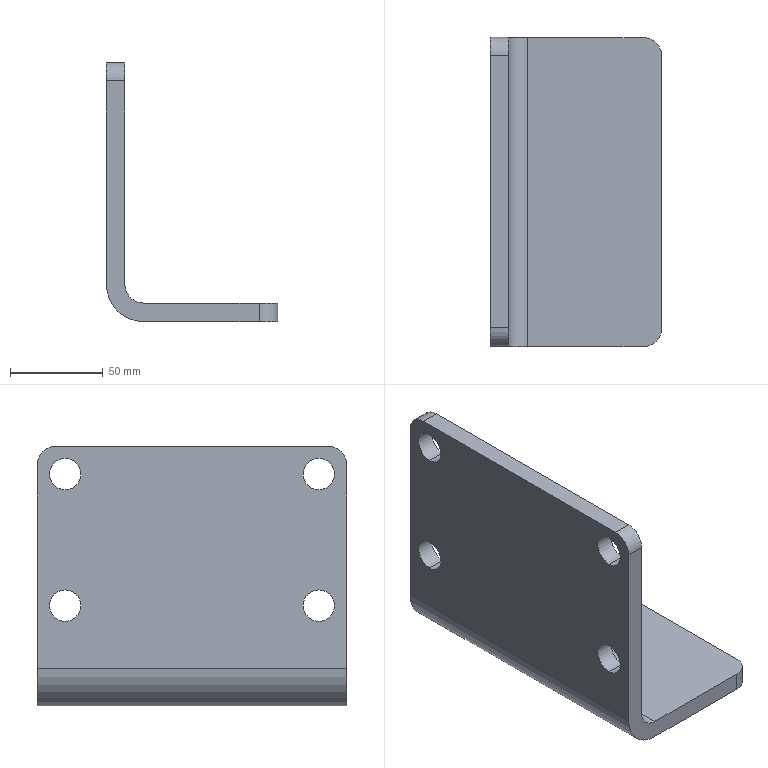Part | STEP file | VD-SYL0380DJ1006_1_4-1_VD-SYL03 | 1 solid | 22 faces | box 92.5 x 167 x 140 mm | volume 350886 mm3 | cylinder 14 | plane 8 | commonest cylinder face diameters 17 x8 20 x5 40 x1
STEP:
#1=CARTESIAN_POINT('',(0.,-152.,-94.5));
#2=VERTEX_POINT('',#1);
#3=CARTESIAN_POINT('',(10.,-152.,-94.5));
#4=VERTEX_POINT('',#3);
#5=CARTESIAN_POINT('',(0.,-152.,-94.5));
#6=DIRECTION('',(1.,0.,0.));
#7=VECTOR('',#6,1000.);
#8=LINE('',#5,#7);
#9=EDGE_CURVE('',#2,#4,#8,.T.);
#10=ORIENTED_EDGE('',*,*,#9,.F.);
#11=CARTESIAN_POINT('',(0.,-152.,-77.5));
#12=VERTEX_POINT('',#11);
#13=CARTESIAN_POINT('',(0.,-152.,-86.));
#14=DIRECTION('',(1.,0.,0.));
#15=DIRECTION('',(0.,0.,1.));
#16=AXIS2_PLACEMENT_3D('',#13,#14,#15);
#17=CIRCLE('',#16,8.5);
#18=EDGE_CURVE('',#12,#2,#17,.T.);
#19=ORIENTED_EDGE('',*,*,#18,.F.);
#20=CARTESIAN_POINT('',(10.,-152.,-77.5));
#21=VERTEX_POINT('',#20);
#22=CARTESIAN_POINT('',(0.,-152.,-77.5));
#23=DIRECTION('',(1.,0.,0.));
#24=VECTOR('',#23,1000.);
#25=LINE('',#22,#24);
#26=EDGE_CURVE('',#12,#21,#25,.T.);
#27=ORIENTED_EDGE('',*,*,#26,.T.);
#28=CARTESIAN_POINT('',(10.,-152.,-86.));
#29=DIRECTION('',(-1.,0.,0.));
#30=DIRECTION('',(0.,0.,-1.));
#31=AXIS2_PLACEMENT_3D('',#28,#29,#30);
#32=CIRCLE('',#31,8.5);
#33=EDGE_CURVE('',#4,#21,#32,.T.);
#34=ORIENTED_EDGE('',*,*,#33,.F.);
#35=EDGE_LOOP('',(#10,#19,#27,#34));
#36=FACE_OUTER_BOUND('',#35,.T.);
#37=CARTESIAN_POINT('',(5.,-152.,-86.));
#38=DIRECTION('',(-1.,0.,0.));
#39=DIRECTION('',(0.,0.,1.));
#40=AXIS2_PLACEMENT_3D('',#37,#38,#39);
#41=CYLINDRICAL_SURFACE('',#40,8.5);
#42=ADVANCED_FACE('',(#36),#41,.F.);
#43=CARTESIAN_POINT('',(10.,-152.,-86.));
#44=DIRECTION('',(-1.,0.,0.));
#45=DIRECTION('',(0.,0.,1.));
#46=AXIS2_PLACEMENT_3D('',#43,#44,#45);
#47=CIRCLE('',#46,8.5);
#48=EDGE_CURVE('',#21,#4,#47,.T.);
#49=ORIENTED_EDGE('',*,*,#48,.F.);
#50=ORIENTED_EDGE('',*,*,#26,.F.);
#51=CARTESIAN_POINT('',(0.,-152.,-86.));
#52=DIRECTION('',(1.,0.,0.));
#53=DIRECTION('',(0.,0.,-1.));
#54=AXIS2_PLACEMENT_3D('',#51,#52,#53);
#55=CIRCLE('',#54,8.5);
#56=EDGE_CURVE('',#2,#12,#55,.T.);
#57=ORIENTED_EDGE('',*,*,#56,.F.);
#58=ORIENTED_EDGE('',*,*,#9,.T.);
#59=EDGE_LOOP('',(#49,#50,#57,#58));
#60=FACE_OUTER_BOUND('',#59,.T.);
#61=CARTESIAN_POINT('',(5.,-152.,-86.));
#62=DIRECTION('',(-1.,0.,0.));
#63=DIRECTION('',(0.,0.,1.));
#64=AXIS2_PLACEMENT_3D('',#61,#62,#63);
#65=CYLINDRICAL_SURFACE('',#64,8.5);
#66=ADVANCED_FACE('',(#60),#65,.F.);
#67=CARTESIAN_POINT('',(0.,-15.,-94.5));
#68=VERTEX_POINT('',#67);
#69=CARTESIAN_POINT('',(10.,-15.,-94.5));
#70=VERTEX_POINT('',#69);
#71=CARTESIAN_POINT('',(0.,-15.,-94.5));
#72=DIRECTION('',(1.,0.,0.));
#73=VECTOR('',#72,1000.);
#74=LINE('',#71,#73);
#75=EDGE_CURVE('',#68,#70,#74,.T.);
#76=ORIENTED_EDGE('',*,*,#75,.F.);
#77=CARTESIAN_POINT('',(0.,-15.,-77.5));
#78=VERTEX_POINT('',#77);
#79=CARTESIAN_POINT('',(0.,-15.,-86.));
#80=DIRECTION('',(1.,0.,0.));
#81=DIRECTION('',(0.,0.,1.));
#82=AXIS2_PLACEMENT_3D('',#79,#80,#81);
#83=CIRCLE('',#82,8.5);
#84=EDGE_CURVE('',#78,#68,#83,.T.);
#85=ORIENTED_EDGE('',*,*,#84,.F.);
#86=CARTESIAN_POINT('',(10.,-15.,-77.5));
#87=VERTEX_POINT('',#86);
#88=CARTESIAN_POINT('',(0.,-15.,-77.5));
#89=DIRECTION('',(1.,0.,0.));
#90=VECTOR('',#89,1000.);
#91=LINE('',#88,#90);
#92=EDGE_CURVE('',#78,#87,#91,.T.);
#93=ORIENTED_EDGE('',*,*,#92,.T.);
#94=CARTESIAN_POINT('',(10.,-15.,-86.));
#95=DIRECTION('',(-1.,0.,0.));
#96=DIRECTION('',(0.,0.,-1.));
#97=AXIS2_PLACEMENT_3D('',#94,#95,#96);
#98=CIRCLE('',#97,8.5);
#99=EDGE_CURVE('',#70,#87,#98,.T.);
#100=ORIENTED_EDGE('',*,*,#99,.F.);
#101=EDGE_LOOP('',(#76,#85,#93,#100));
#102=FACE_OUTER_BOUND('',#101,.T.);
#103=CARTESIAN_POINT('',(5.,-15.,-86.));
#104=DIRECTION('',(-1.,0.,0.));
#105=DIRECTION('',(0.,0.,1.));
#106=AXIS2_PLACEMENT_3D('',#103,#104,#105);
#107=CYLINDRICAL_SURFACE('',#106,8.5);
#108=ADVANCED_FACE('',(#102),#107,.F.);
#109=CARTESIAN_POINT('',(10.,-15.,-86.));
#110=DIRECTION('',(-1.,0.,0.));
#111=DIRECTION('',(0.,0.,1.));
#112=AXIS2_PLACEMENT_3D('',#109,#110,#111);
#113=CIRCLE('',#112,8.5);
#114=EDGE_CURVE('',#87,#70,#113,.T.);
#115=ORIENTED_EDGE('',*,*,#114,.F.);
#116=ORIENTED_EDGE('',*,*,#92,.F.);
#117=CARTESIAN_POINT('',(0.,-15.,-86.));
#118=DIRECTION('',(1.,0.,0.));
#119=DIRECTION('',(0.,0.,-1.));
#120=AXIS2_PLACEMENT_3D('',#117,#118,#119);
#121=CIRCLE('',#120,8.5);
#122=EDGE_CURVE('',#68,#78,#121,.T.);
#123=ORIENTED_EDGE('',*,*,#122,.F.);
#124=ORIENTED_EDGE('',*,*,#75,.T.);
#125=EDGE_LOOP('',(#115,#116,#123,#124));
#126=FACE_OUTER_BOUND('',#125,.T.);
#127=CARTESIAN_POINT('',(5.,-15.,-86.));
#128=DIRECTION('',(-1.,0.,0.));
#129=DIRECTION('',(0.,0.,1.));
#130=AXIS2_PLACEMENT_3D('',#127,#128,#129);
#131=CYLINDRICAL_SURFACE('',#130,8.5);
#132=ADVANCED_FACE('',(#126),#131,.F.);
#133=CARTESIAN_POINT('',(0.,-152.,-23.5));
#134=VERTEX_POINT('',#133);
#135=CARTESIAN_POINT('',(10.,-152.,-23.5));
#136=VERTEX_POINT('',#135);
#137=CARTESIAN_POINT('',(0.,-152.,-23.5));
#138=DIRECTION('',(1.,0.,0.));
#139=VECTOR('',#138,1000.);
#140=LINE('',#137,#139);
#141=EDGE_CURVE('',#134,#136,#140,.T.);
#142=ORIENTED_EDGE('',*,*,#141,.F.);
#143=CARTESIAN_POINT('',(0.,-152.,-6.5));
#144=VERTEX_POINT('',#143);
#145=CARTESIAN_POINT('',(0.,-152.,-15.));
#146=DIRECTION('',(1.,0.,0.));
#147=DIRECTION('',(0.,0.,1.));
#148=AXIS2_PLACEMENT_3D('',#145,#146,#147);
#149=CIRCLE('',#148,8.5);
#150=EDGE_CURVE('',#144,#134,#149,.T.);
#151=ORIENTED_EDGE('',*,*,#150,.F.);
#152=CARTESIAN_POINT('',(10.,-152.,-6.5));
#153=VERTEX_POINT('',#152);
#154=CARTESIAN_POINT('',(0.,-152.,-6.5));
#155=DIRECTION('',(1.,0.,0.));
#156=VECTOR('',#155,1000.);
#157=LINE('',#154,#156);
#158=EDGE_CURVE('',#144,#153,#157,.T.);
#159=ORIENTED_EDGE('',*,*,#158,.T.);
#160=CARTESIAN_POINT('',(10.,-152.,-15.));
#161=DIRECTION('',(-1.,0.,0.));
#162=DIRECTION('',(0.,0.,-1.));
#163=AXIS2_PLACEMENT_3D('',#160,#161,#162);
#164=CIRCLE('',#163,8.5);
#165=EDGE_CURVE('',#136,#153,#164,.T.);
#166=ORIENTED_EDGE('',*,*,#165,.F.);
#167=EDGE_LOOP('',(#142,#151,#159,#166));
#168=FACE_OUTER_BOUND('',#167,.T.);
#169=CARTESIAN_POINT('',(5.,-152.,-15.));
#170=DIRECTION('',(-1.,0.,0.));
#171=DIRECTION('',(0.,0.,1.));
#172=AXIS2_PLACEMENT_3D('',#169,#170,#171);
#173=CYLINDRICAL_SURFACE('',#172,8.5);
#174=ADVANCED_FACE('',(#168),#173,.F.);
#175=CARTESIAN_POINT('',(10.,-152.,-15.));
#176=DIRECTION('',(-1.,0.,0.));
#177=DIRECTION('',(0.,0.,1.));
#178=AXIS2_PLACEMENT_3D('',#175,#176,#177);
#179=CIRCLE('',#178,8.5);
#180=EDGE_CURVE('',#153,#136,#179,.T.);
#181=ORIENTED_EDGE('',*,*,#180,.F.);
#182=ORIENTED_EDGE('',*,*,#158,.F.);
#183=CARTESIAN_POINT('',(0.,-152.,-15.));
#184=DIRECTION('',(1.,0.,0.));
#185=DIRECTION('',(0.,0.,-1.));
#186=AXIS2_PLACEMENT_3D('',#183,#184,#185);
#187=CIRCLE('',#186,8.5);
#188=EDGE_CURVE('',#134,#144,#187,.T.);
#189=ORIENTED_EDGE('',*,*,#188,.F.);
#190=ORIENTED_EDGE('',*,*,#141,.T.);
#191=EDGE_LOOP('',(#181,#182,#189,#190));
#192=FACE_OUTER_BOUND('',#191,.T.);
#193=CARTESIAN_POINT('',(5.,-152.,-15.));
#194=DIRECTION('',(-1.,0.,0.));
#195=DIRECTION('',(0.,0.,1.));
#196=AXIS2_PLACEMENT_3D('',#193,#194,#195);
#197=CYLINDRICAL_SURFACE('',#196,8.5);
#198=ADVANCED_FACE('',(#192),#197,.F.);
#199=CARTESIAN_POINT('',(0.,-15.,-23.5));
#200=VERTEX_POINT('',#199);
#201=CARTESIAN_POINT('',(10.,-15.,-23.5));
#202=VERTEX_POINT('',#201);
#203=CARTESIAN_POINT('',(0.,-15.,-23.5));
#204=DIRECTION('',(1.,0.,0.));
#205=VECTOR('',#204,1000.);
#206=LINE('',#203,#205);
#207=EDGE_CURVE('',#200,#202,#206,.T.);
#208=ORIENTED_EDGE('',*,*,#207,.F.);
#209=CARTESIAN_POINT('',(0.,-15.,-6.5));
#210=VERTEX_POINT('',#209);
#211=CARTESIAN_POINT('',(0.,-15.,-15.));
#212=DIRECTION('',(1.,0.,0.));
#213=DIRECTION('',(0.,0.,1.));
#214=AXIS2_PLACEMENT_3D('',#211,#212,#213);
#215=CIRCLE('',#214,8.5);
#216=EDGE_CURVE('',#210,#200,#215,.T.);
#217=ORIENTED_EDGE('',*,*,#216,.F.);
#218=CARTESIAN_POINT('',(10.,-15.,-6.5));
#219=VERTEX_POINT('',#218);
#220=CARTESIAN_POINT('',(0.,-15.,-6.5));
#221=DIRECTION('',(1.,0.,0.));
#222=VECTOR('',#221,1000.);
#223=LINE('',#220,#222);
#224=EDGE_CURVE('',#210,#219,#223,.T.);
#225=ORIENTED_EDGE('',*,*,#224,.T.);
#226=CARTESIAN_POINT('',(10.,-15.,-15.));
#227=DIRECTION('',(-1.,0.,0.));
#228=DIRECTION('',(0.,0.,-1.));
#229=AXIS2_PLACEMENT_3D('',#226,#227,#228);
#230=CIRCLE('',#229,8.5);
#231=EDGE_CURVE('',#202,#219,#230,.T.);
#232=ORIENTED_EDGE('',*,*,#231,.F.);
#233=EDGE_LOOP('',(#208,#217,#225,#232));
#234=FACE_OUTER_BOUND('',#233,.T.);
#235=CARTESIAN_POINT('',(5.,-15.,-15.));
#236=DIRECTION('',(-1.,0.,0.));
#237=DIRECTION('',(0.,0.,1.));
#238=AXIS2_PLACEMENT_3D('',#235,#236,#237);
#239=CYLINDRICAL_SURFACE('',#238,8.5);
#240=ADVANCED_FACE('',(#234),#239,.F.);
#241=CARTESIAN_POINT('',(10.,-15.,-15.));
#242=DIRECTION('',(-1.,0.,0.));
#243=DIRECTION('',(0.,0.,1.));
#244=AXIS2_PLACEMENT_3D('',#241,#242,#243);
#245=CIRCLE('',#244,8.5);
#246=EDGE_CURVE('',#219,#202,#245,.T.);
#247=ORIENTED_EDGE('',*,*,#246,.F.);
#248=ORIENTED_EDGE('',*,*,#224,.F.);
#249=CARTESIAN_POINT('',(0.,-15.,-15.));
#250=DIRECTION('',(1.,0.,0.));
#251=DIRECTION('',(0.,0.,-1.));
#252=AXIS2_PLACEMENT_3D('',#249,#250,#251);
#253=CIRCLE('',#252,8.5);
#254=EDGE_CURVE('',#200,#210,#253,.T.);
#255=ORIENTED_EDGE('',*,*,#254,.F.);
#256=ORIENTED_EDGE('',*,*,#207,.T.);
#257=EDGE_LOOP('',(#247,#248,#255,#256));
#258=FACE_OUTER_BOUND('',#257,.T.);
#259=CARTESIAN_POINT('',(5.,-15.,-15.));
#260=DIRECTION('',(-1.,0.,0.));
#261=DIRECTION('',(0.,0.,1.));
#262=AXIS2_PLACEMENT_3D('',#259,#260,#261);
#263=CYLINDRICAL_SURFACE('',#262,8.5);
#264=ADVANCED_FACE('',(#258),#263,.F.);
#265=ORIENTED_EDGE('',*,*,#33,.T.);
#266=ORIENTED_EDGE('',*,*,#48,.T.);
#267=EDGE_LOOP('',(#265,#266));
#268=FACE_BOUND('',#267,.T.);
#269=ORIENTED_EDGE('',*,*,#99,.T.);
#270=ORIENTED_EDGE('',*,*,#114,.T.);
#271=EDGE_LOOP('',(#269,#270));
#272=FACE_BOUND('',#271,.T.);
#273=ORIENTED_EDGE('',*,*,#165,.T.);
#274=ORIENTED_EDGE('',*,*,#180,.T.);
#275=EDGE_LOOP('',(#273,#274));
#276=FACE_BOUND('',#275,.T.);
#277=ORIENTED_EDGE('',*,*,#231,.T.);
#278=ORIENTED_EDGE('',*,*,#246,.T.);
#279=EDGE_LOOP('',(#277,#278));
#280=FACE_BOUND('',#279,.T.);
#281=CARTESIAN_POINT('',(10.,0.,-120.));
#282=VERTEX_POINT('',#281);
#283=CARTESIAN_POINT('',(10.,-167.,-120.));
#284=VERTEX_POINT('',#283);
#285=CARTESIAN_POINT('',(10.,0.,-120.));
#286=DIRECTION('',(0.,-1.,0.));
#287=VECTOR('',#286,1000.);
#288=LINE('',#285,#287);
#289=EDGE_CURVE('',#282,#284,#288,.T.);
#290=ORIENTED_EDGE('',*,*,#289,.F.);
#291=CARTESIAN_POINT('',(10.,0.,-10.));
#292=VERTEX_POINT('',#291);
#293=CARTESIAN_POINT('',(10.,0.,-10.));
#294=DIRECTION('',(0.,0.,-1.));
#295=VECTOR('',#294,1000.);
#296=LINE('',#293,#295);
#297=EDGE_CURVE('',#292,#282,#296,.T.);
#298=ORIENTED_EDGE('',*,*,#297,.F.);
#299=CARTESIAN_POINT('',(10.,-10.,0.));
#300=VERTEX_POINT('',#299);
#301=CARTESIAN_POINT('',(10.,-10.,-10.));
#302=DIRECTION('',(1.,0.,0.));
#303=DIRECTION('',(0.,1.,0.));
#304=AXIS2_PLACEMENT_3D('',#301,#302,#303);
#305=CIRCLE('',#304,10.);
#306=EDGE_CURVE('',#292,#300,#305,.T.);
#307=ORIENTED_EDGE('',*,*,#306,.T.);
#308=CARTESIAN_POINT('',(10.,-157.,0.));
#309=VERTEX_POINT('',#308);
#310=CARTESIAN_POINT('',(10.,-157.,0.));
#311=DIRECTION('',(0.,1.,0.));
#312=VECTOR('',#311,1000.);
#313=LINE('',#310,#312);
#314=EDGE_CURVE('',#309,#300,#313,.T.);
#315=ORIENTED_EDGE('',*,*,#314,.F.);
#316=CARTESIAN_POINT('',(10.,-167.,-10.));
#317=VERTEX_POINT('',#316);
#318=CARTESIAN_POINT('',(10.,-157.,-10.));
#319=DIRECTION('',(1.,0.,0.));
#320=DIRECTION('',(0.,0.,1.));
#321=AXIS2_PLACEMENT_3D('',#318,#319,#320);
#322=CIRCLE('',#321,10.);
#323=EDGE_CURVE('',#309,#317,#322,.T.);
#324=ORIENTED_EDGE('',*,*,#323,.T.);
#325=CARTESIAN_POINT('',(10.,-167.,-120.));
#326=DIRECTION('',(0.,0.,1.));
#327=VECTOR('',#326,1000.);
#328=LINE('',#325,#327);
#329=EDGE_CURVE('',#284,#317,#328,.T.);
#330=ORIENTED_EDGE('',*,*,#329,.F.);
#331=EDGE_LOOP('',(#290,#298,#307,#315,#324,#330));
#332=FACE_OUTER_BOUND('',#331,.T.);
#333=CARTESIAN_POINT('',(10.,0.,0.));
#334=DIRECTION('',(1.,0.,0.));
#335=DIRECTION('',(0.,1.,0.));
#336=AXIS2_PLACEMENT_3D('',#333,#334,#335);
#337=PLANE('',#336);
#338=ADVANCED_FACE('',(#268,#272,#276,#280,#332),#337,.T.);
#339=CARTESIAN_POINT('',(20.,0.,-130.));
#340=VERTEX_POINT('',#339);
#341=CARTESIAN_POINT('',(20.,0.,-120.));
#342=DIRECTION('',(0.,-1.,0.));
#343=DIRECTION('',(-1.,0.,0.));
#344=AXIS2_PLACEMENT_3D('',#341,#342,#343);
#345=CIRCLE('',#344,10.);
#346=EDGE_CURVE('',#282,#340,#345,.T.);
#347=ORIENTED_EDGE('',*,*,#346,.F.);
#348=ORIENTED_EDGE('',*,*,#289,.T.);
#349=CARTESIAN_POINT('',(20.,-167.,-130.));
#350=VERTEX_POINT('',#349);
#351=CARTESIAN_POINT('',(20.,-167.,-120.));
#352=DIRECTION('',(0.,1.,0.));
#353=DIRECTION('',(0.,0.,-1.));
#354=AXIS2_PLACEMENT_3D('',#351,#352,#353);
#355=CIRCLE('',#354,10.);
#356=EDGE_CURVE('',#350,#284,#355,.T.);
#357=ORIENTED_EDGE('',*,*,#356,.F.);
#358=CARTESIAN_POINT('',(20.,-167.,-130.));
#359=DIRECTION('',(0.,1.,0.));
#360=VECTOR('',#359,1000.);
#361=LINE('',#358,#360);
#362=EDGE_CURVE('',#350,#340,#361,.T.);
#363=ORIENTED_EDGE('',*,*,#362,.T.);
#364=EDGE_LOOP('',(#347,#348,#357,#363));
#365=FACE_OUTER_BOUND('',#364,.T.);
#366=CARTESIAN_POINT('',(20.,217.701,-120.));
#367=DIRECTION('',(0.,-1.,0.));
#368=DIRECTION('',(0.,0.,-1.));
#369=AXIS2_PLACEMENT_3D('',#366,#367,#368);
#370=CYLINDRICAL_SURFACE('',#369,10.);
#371=ADVANCED_FACE('',(#365),#370,.F.);
#372=ORIENTED_EDGE('',*,*,#362,.F.);
#373=CARTESIAN_POINT('',(82.5,-167.,-130.));
#374=VERTEX_POINT('',#373);
#375=CARTESIAN_POINT('',(82.5,-167.,-130.));
#376=DIRECTION('',(-1.,0.,0.));
#377=VECTOR('',#376,1000.);
#378=LINE('',#375,#377);
#379=EDGE_CURVE('',#374,#350,#378,.T.);
#380=ORIENTED_EDGE('',*,*,#379,.F.);
#381=CARTESIAN_POINT('',(92.5,-157.,-130.));
#382=VERTEX_POINT('',#381);
#383=CARTESIAN_POINT('',(82.5,-157.,-130.));
#384=DIRECTION('',(0.,0.,1.));
#385=DIRECTION('',(0.,-1.,0.));
#386=AXIS2_PLACEMENT_3D('',#383,#384,#385);
#387=CIRCLE('',#386,10.);
#388=EDGE_CURVE('',#374,#382,#387,.T.);
#389=ORIENTED_EDGE('',*,*,#388,.T.);
#390=CARTESIAN_POINT('',(92.5,-10.,-130.));
#391=VERTEX_POINT('',#390);
#392=CARTESIAN_POINT('',(92.5,-10.,-130.));
#393=DIRECTION('',(0.,-1.,0.));
#394=VECTOR('',#393,1000.);
#395=LINE('',#392,#394);
#396=EDGE_CURVE('',#391,#382,#395,.T.);
#397=ORIENTED_EDGE('',*,*,#396,.F.);
#398=CARTESIAN_POINT('',(82.5,0.,-130.));
#399=VERTEX_POINT('',#398);
#400=CARTESIAN_POINT('',(82.5,-10.,-130.));
#401=DIRECTION('',(0.,0.,1.));
#402=DIRECTION('',(1.,0.,0.));
#403=AXIS2_PLACEMENT_3D('',#400,#401,#402);
#404=CIRCLE('',#403,10.);
#405=EDGE_CURVE('',#391,#399,#404,.T.);
#406=ORIENTED_EDGE('',*,*,#405,.T.);
#407=CARTESIAN_POINT('',(20.,0.,-130.));
#408=DIRECTION('',(1.,0.,0.));
#409=VECTOR('',#408,1000.);
#410=LINE('',#407,#409);
#411=EDGE_CURVE('',#340,#399,#410,.T.);
#412=ORIENTED_EDGE('',*,*,#411,.F.);
#413=EDGE_LOOP('',(#372,#380,#389,#397,#406,#412));
#414=FACE_OUTER_BOUND('',#413,.T.);
#415=CARTESIAN_POINT('',(10.,0.,-130.));
#416=DIRECTION('',(0.,0.,1.));
#417=DIRECTION('',(1.,0.,0.));
#418=AXIS2_PLACEMENT_3D('',#415,#416,#417);
#419=PLANE('',#418);
#420=ADVANCED_FACE('',(#414),#419,.T.);
#421=CARTESIAN_POINT('',(92.5,-10.,-140.));
#422=VERTEX_POINT('',#421);
#423=CARTESIAN_POINT('',(92.5,-10.,-130.));
#424=DIRECTION('',(0.,0.,-1.));
#425=VECTOR('',#424,1000.);
#426=LINE('',#423,#425);
#427=EDGE_CURVE('',#391,#422,#426,.T.);
#428=ORIENTED_EDGE('',*,*,#427,.F.);
#429=ORIENTED_EDGE('',*,*,#396,.T.);
#430=CARTESIAN_POINT('',(92.5,-157.,-140.));
#431=VERTEX_POINT('',#430);
#432=CARTESIAN_POINT('',(92.5,-157.,-140.));
#433=DIRECTION('',(0.,0.,1.));
#434=VECTOR('',#433,1000.);
#435=LINE('',#432,#434);
#436=EDGE_CURVE('',#431,#382,#435,.T.);
#437=ORIENTED_EDGE('',*,*,#436,.F.);
#438=CARTESIAN_POINT('',(92.5,-157.,-140.));
#439=DIRECTION('',(0.,1.,0.));
#440=VECTOR('',#439,1000.);
#441=LINE('',#438,#440);
#442=EDGE_CURVE('',#431,#422,#441,.T.);
#443=ORIENTED_EDGE('',*,*,#442,.T.);
#444=EDGE_LOOP('',(#428,#429,#437,#443));
#445=FACE_OUTER_BOUND('',#444,.T.);
#446=CARTESIAN_POINT('',(92.5,-83.5,-135.));
#447=DIRECTION('',(-1.,0.,0.));
#448=DIRECTION('',(0.,0.,1.));
#449=AXIS2_PLACEMENT_3D('',#446,#447,#448);
#450=PLANE('',#449);
#451=ADVANCED_FACE('',(#445),#450,.F.);
#452=ORIENTED_EDGE('',*,*,#388,.F.);
#453=CARTESIAN_POINT('',(82.5,-167.,-140.));
#454=VERTEX_POINT('',#453);
#455=CARTESIAN_POINT('',(82.5,-167.,-130.));
#456=DIRECTION('',(0.,0.,-1.));
#457=VECTOR('',#456,1000.);
#458=LINE('',#455,#457);
#459=EDGE_CURVE('',#374,#454,#458,.T.);
#460=ORIENTED_EDGE('',*,*,#459,.T.);
#461=CARTESIAN_POINT('',(82.5,-157.,-140.));
#462=DIRECTION('',(0.,0.,-1.));
#463=DIRECTION('',(1.,0.,0.));
#464=AXIS2_PLACEMENT_3D('',#461,#462,#463);
#465=CIRCLE('',#464,10.);
#466=EDGE_CURVE('',#431,#454,#465,.T.);
#467=ORIENTED_EDGE('',*,*,#466,.F.);
#468=ORIENTED_EDGE('',*,*,#436,.T.);
#469=EDGE_LOOP('',(#452,#460,#467,#468));
#470=FACE_OUTER_BOUND('',#469,.T.);
#471=CARTESIAN_POINT('',(82.5,-157.,-135.));
#472=DIRECTION('',(0.,0.,1.));
#473=DIRECTION('',(1.,0.,0.));
#474=AXIS2_PLACEMENT_3D('',#471,#472,#473);
#475=CYLINDRICAL_SURFACE('',#474,10.);
#476=ADVANCED_FACE('',(#470),#475,.T.);
#477=ORIENTED_EDGE('',*,*,#442,.F.);
#478=ORIENTED_EDGE('',*,*,#466,.T.);
#479=CARTESIAN_POINT('',(20.,-167.,-140.));
#480=VERTEX_POINT('',#479);
#481=CARTESIAN_POINT('',(82.5,-167.,-140.));
#482=DIRECTION('',(-1.,0.,0.));
#483=VECTOR('',#482,1000.);
#484=LINE('',#481,#483);
#485=EDGE_CURVE('',#454,#480,#484,.T.);
#486=ORIENTED_EDGE('',*,*,#485,.T.);
#487=CARTESIAN_POINT('',(20.,0.,-140.));
#488=VERTEX_POINT('',#487);
#489=CARTESIAN_POINT('',(20.,0.,-140.));
#490=DIRECTION('',(0.,-1.,0.));
#491=VECTOR('',#490,1000.);
#492=LINE('',#489,#491);
#493=EDGE_CURVE('',#488,#480,#492,.T.);
#494=ORIENTED_EDGE('',*,*,#493,.F.);
#495=CARTESIAN_POINT('',(82.5,0.,-140.));
#496=VERTEX_POINT('',#495);
#497=CARTESIAN_POINT('',(82.5,0.,-140.));
#498=DIRECTION('',(-1.,0.,0.));
#499=VECTOR('',#498,1000.);
#500=LINE('',#497,#499);
#501=EDGE_CURVE('',#496,#488,#500,.T.);
#502=ORIENTED_EDGE('',*,*,#501,.F.);
#503=CARTESIAN_POINT('',(82.5,-10.,-140.));
#504=DIRECTION('',(0.,0.,-1.));
#505=DIRECTION('',(0.,1.,0.));
#506=AXIS2_PLACEMENT_3D('',#503,#504,#505);
#507=CIRCLE('',#506,10.);
#508=EDGE_CURVE('',#496,#422,#507,.T.);
#509=ORIENTED_EDGE('',*,*,#508,.T.);
#510=EDGE_LOOP('',(#477,#478,#486,#494,#502,#509));
#511=FACE_OUTER_BOUND('',#510,.T.);
#512=CARTESIAN_POINT('',(10.,0.,-140.));
#513=DIRECTION('',(0.,0.,1.));
#514=DIRECTION('',(1.,0.,0.));
#515=AXIS2_PLACEMENT_3D('',#512,#513,#514);
#516=PLANE('',#515);
#517=ADVANCED_FACE('',(#511),#516,.F.);
#518=CARTESIAN_POINT('',(0.,-167.,-120.));
#519=VERTEX_POINT('',#518);
#520=CARTESIAN_POINT('',(0.,0.,-120.));
#521=VERTEX_POINT('',#520);
#522=CARTESIAN_POINT('',(0.,-167.,-120.));
#523=DIRECTION('',(0.,1.,0.));
#524=VECTOR('',#523,1000.);
#525=LINE('',#522,#524);
#526=EDGE_CURVE('',#519,#521,#525,.T.);
#527=ORIENTED_EDGE('',*,*,#526,.T.);
#528=CARTESIAN_POINT('',(20.,0.,-120.));
#529=DIRECTION('',(0.,1.,0.));
#530=DIRECTION('',(0.,0.,-1.));
#531=AXIS2_PLACEMENT_3D('',#528,#529,#530);
#532=CIRCLE('',#531,20.);
#533=EDGE_CURVE('',#488,#521,#532,.T.);
#534=ORIENTED_EDGE('',*,*,#533,.F.);
#535=ORIENTED_EDGE('',*,*,#493,.T.);
#536=CARTESIAN_POINT('',(20.,-167.,-120.));
#537=DIRECTION('',(0.,-1.,0.));
#538=DIRECTION('',(-1.,0.,0.));
#539=AXIS2_PLACEMENT_3D('',#536,#537,#538);
#540=CIRCLE('',#539,20.);
#541=EDGE_CURVE('',#519,#480,#540,.T.);
#542=ORIENTED_EDGE('',*,*,#541,.F.);
#543=EDGE_LOOP('',(#527,#534,#535,#542));
#544=FACE_OUTER_BOUND('',#543,.T.);
#545=CARTESIAN_POINT('',(20.,217.701,-120.));
#546=DIRECTION('',(0.,-1.,0.));
#547=DIRECTION('',(0.,0.,-1.));
#548=AXIS2_PLACEMENT_3D('',#545,#546,#547);
#549=CYLINDRICAL_SURFACE('',#548,20.);
#550=ADVANCED_FACE('',(#544),#549,.T.);
#551=ORIENTED_EDGE('',*,*,#56,.T.);
#552=ORIENTED_EDGE('',*,*,#18,.T.);
#553=EDGE_LOOP('',(#551,#552));
#554=FACE_BOUND('',#553,.T.);
#555=ORIENTED_EDGE('',*,*,#122,.T.);
#556=ORIENTED_EDGE('',*,*,#84,.T.);
#557=EDGE_LOOP('',(#555,#556));
#558=FACE_BOUND('',#557,.T.);
#559=ORIENTED_EDGE('',*,*,#188,.T.);
#560=ORIENTED_EDGE('',*,*,#150,.T.);
#561=EDGE_LOOP('',(#559,#560));
#562=FACE_BOUND('',#561,.T.);
#563=ORIENTED_EDGE('',*,*,#254,.T.);
#564=ORIENTED_EDGE('',*,*,#216,.T.);
#565=EDGE_LOOP('',(#563,#564));
#566=FACE_BOUND('',#565,.T.);
#567=CARTESIAN_POINT('',(0.,-157.,0.));
#568=VERTEX_POINT('',#567);
#569=CARTESIAN_POINT('',(0.,-10.,0.));
#570=VERTEX_POINT('',#569);
#571=CARTESIAN_POINT('',(0.,-157.,0.));
#572=DIRECTION('',(0.,1.,0.));
#573=VECTOR('',#572,1000.);
#574=LINE('',#571,#573);
#575=EDGE_CURVE('',#568,#570,#574,.T.);
#576=ORIENTED_EDGE('',*,*,#575,.T.);
#577=CARTESIAN_POINT('',(0.,0.,-10.));
#578=VERTEX_POINT('',#577);
#579=CARTESIAN_POINT('',(0.,-10.,-10.));
#580=DIRECTION('',(-1.,0.,0.));
#581=DIRECTION('',(0.,0.,1.));
#582=AXIS2_PLACEMENT_3D('',#579,#580,#581);
#583=CIRCLE('',#582,10.);
#584=EDGE_CURVE('',#570,#578,#583,.T.);
#585=ORIENTED_EDGE('',*,*,#584,.T.);
#586=CARTESIAN_POINT('',(0.,0.,-10.));
#587=DIRECTION('',(0.,0.,-1.));
#588=VECTOR('',#587,1000.);
#589=LINE('',#586,#588);
#590=EDGE_CURVE('',#578,#521,#589,.T.);
#591=ORIENTED_EDGE('',*,*,#590,.T.);
#592=ORIENTED_EDGE('',*,*,#526,.F.);
#593=CARTESIAN_POINT('',(0.,-167.,-10.));
#594=VERTEX_POINT('',#593);
#595=CARTESIAN_POINT('',(0.,-167.,-120.));
#596=DIRECTION('',(0.,0.,1.));
#597=VECTOR('',#596,1000.);
#598=LINE('',#595,#597);
#599=EDGE_CURVE('',#519,#594,#598,.T.);
#600=ORIENTED_EDGE('',*,*,#599,.T.);
#601=CARTESIAN_POINT('',(0.,-157.,-10.));
#602=DIRECTION('',(-1.,0.,0.));
#603=DIRECTION('',(0.,-1.,0.));
#604=AXIS2_PLACEMENT_3D('',#601,#602,#603);
#605=CIRCLE('',#604,10.);
#606=EDGE_CURVE('',#594,#568,#605,.T.);
#607=ORIENTED_EDGE('',*,*,#606,.T.);
#608=EDGE_LOOP('',(#576,#585,#591,#592,#600,#607));
#609=FACE_OUTER_BOUND('',#608,.T.);
#610=CARTESIAN_POINT('',(0.,0.,0.));
#611=DIRECTION('',(1.,0.,0.));
#612=DIRECTION('',(0.,1.,0.));
#613=AXIS2_PLACEMENT_3D('',#610,#611,#612);
#614=PLANE('',#613);
#615=ADVANCED_FACE('',(#554,#558,#562,#566,#609),#614,.F.);
#616=ORIENTED_EDGE('',*,*,#541,.T.);
#617=ORIENTED_EDGE('',*,*,#485,.F.);
#618=ORIENTED_EDGE('',*,*,#459,.F.);
#619=ORIENTED_EDGE('',*,*,#379,.T.);
#620=ORIENTED_EDGE('',*,*,#356,.T.);
#621=ORIENTED_EDGE('',*,*,#329,.T.);
#622=CARTESIAN_POINT('',(0.,-167.,-10.));
#623=DIRECTION('',(1.,0.,0.));
#624=VECTOR('',#623,1000.);
#625=LINE('',#622,#624);
#626=EDGE_CURVE('',#594,#317,#625,.T.);
#627=ORIENTED_EDGE('',*,*,#626,.F.);
#628=ORIENTED_EDGE('',*,*,#599,.F.);
#629=EDGE_LOOP('',(#616,#617,#618,#619,#620,#621,#627,#628));
#630=FACE_OUTER_BOUND('',#629,.T.);
#631=CARTESIAN_POINT('',(5.,-167.,-65.));
#632=DIRECTION('',(0.,-1.,0.));
#633=DIRECTION('',(0.,0.,-1.));
#634=AXIS2_PLACEMENT_3D('',#631,#632,#633);
#635=PLANE('',#634);
#636=ADVANCED_FACE('',(#630),#635,.T.);
#637=ORIENTED_EDGE('',*,*,#323,.F.);
#638=CARTESIAN_POINT('',(10.,-157.,0.));
#639=DIRECTION('',(-1.,0.,0.));
#640=VECTOR('',#639,1000.);
#641=LINE('',#638,#640);
#642=EDGE_CURVE('',#309,#568,#641,.T.);
#643=ORIENTED_EDGE('',*,*,#642,.T.);
#644=ORIENTED_EDGE('',*,*,#606,.F.);
#645=ORIENTED_EDGE('',*,*,#626,.T.);
#646=EDGE_LOOP('',(#637,#643,#644,#645));
#647=FACE_OUTER_BOUND('',#646,.T.);
#648=CARTESIAN_POINT('',(5.,-157.,-10.));
#649=DIRECTION('',(1.,0.,0.));
#650=DIRECTION('',(0.,0.,-1.));
#651=AXIS2_PLACEMENT_3D('',#648,#649,#650);
#652=CYLINDRICAL_SURFACE('',#651,10.);
#653=ADVANCED_FACE('',(#647),#652,.T.);
#654=ORIENTED_EDGE('',*,*,#314,.T.);
#655=CARTESIAN_POINT('',(0.,-10.,0.));
#656=DIRECTION('',(1.,0.,0.));
#657=VECTOR('',#656,1000.);
#658=LINE('',#655,#657);
#659=EDGE_CURVE('',#570,#300,#658,.T.);
#660=ORIENTED_EDGE('',*,*,#659,.F.);
#661=ORIENTED_EDGE('',*,*,#575,.F.);
#662=ORIENTED_EDGE('',*,*,#642,.F.);
#663=EDGE_LOOP('',(#654,#660,#661,#662));
#664=FACE_OUTER_BOUND('',#663,.T.);
#665=CARTESIAN_POINT('',(5.,-83.5,0.));
#666=DIRECTION('',(0.,0.,1.));
#667=DIRECTION('',(1.,0.,0.));
#668=AXIS2_PLACEMENT_3D('',#665,#666,#667);
#669=PLANE('',#668);
#670=ADVANCED_FACE('',(#664),#669,.T.);
#671=ORIENTED_EDGE('',*,*,#306,.F.);
#672=CARTESIAN_POINT('',(10.,0.,-10.));
#673=DIRECTION('',(-1.,0.,0.));
#674=VECTOR('',#673,1000.);
#675=LINE('',#672,#674);
#676=EDGE_CURVE('',#292,#578,#675,.T.);
#677=ORIENTED_EDGE('',*,*,#676,.T.);
#678=ORIENTED_EDGE('',*,*,#584,.F.);
#679=ORIENTED_EDGE('',*,*,#659,.T.);
#680=EDGE_LOOP('',(#671,#677,#678,#679));
#681=FACE_OUTER_BOUND('',#680,.T.);
#682=CARTESIAN_POINT('',(5.,-10.,-10.));
#683=DIRECTION('',(1.,0.,0.));
#684=DIRECTION('',(0.,0.,-1.));
#685=AXIS2_PLACEMENT_3D('',#682,#683,#684);
#686=CYLINDRICAL_SURFACE('',#685,10.);
#687=ADVANCED_FACE('',(#681),#686,.T.);
#688=ORIENTED_EDGE('',*,*,#297,.T.);
#689=ORIENTED_EDGE('',*,*,#346,.T.);
#690=ORIENTED_EDGE('',*,*,#411,.T.);
#691=CARTESIAN_POINT('',(82.5,0.,-140.));
#692=DIRECTION('',(0.,0.,1.));
#693=VECTOR('',#692,1000.);
#694=LINE('',#691,#693);
#695=EDGE_CURVE('',#496,#399,#694,.T.);
#696=ORIENTED_EDGE('',*,*,#695,.F.);
#697=ORIENTED_EDGE('',*,*,#501,.T.);
#698=ORIENTED_EDGE('',*,*,#533,.T.);
#699=ORIENTED_EDGE('',*,*,#590,.F.);
#700=ORIENTED_EDGE('',*,*,#676,.F.);
#701=EDGE_LOOP('',(#688,#689,#690,#696,#697,#698,#699,#700));
#702=FACE_OUTER_BOUND('',#701,.T.);
#703=CARTESIAN_POINT('',(5.,0.,-65.));
#704=DIRECTION('',(0.,1.,0.));
#705=DIRECTION('',(1.,0.,0.));
#706=AXIS2_PLACEMENT_3D('',#703,#704,#705);
#707=PLANE('',#706);
#708=ADVANCED_FACE('',(#702),#707,.T.);
#709=ORIENTED_EDGE('',*,*,#405,.F.);
#710=ORIENTED_EDGE('',*,*,#427,.T.);
#711=ORIENTED_EDGE('',*,*,#508,.F.);
#712=ORIENTED_EDGE('',*,*,#695,.T.);
#713=EDGE_LOOP('',(#709,#710,#711,#712));
#714=FACE_OUTER_BOUND('',#713,.T.);
#715=CARTESIAN_POINT('',(82.5,-10.,-135.));
#716=DIRECTION('',(0.,0.,1.));
#717=DIRECTION('',(1.,0.,0.));
#718=AXIS2_PLACEMENT_3D('',#715,#716,#717);
#719=CYLINDRICAL_SURFACE('',#718,10.);
#720=ADVANCED_FACE('',(#714),#719,.T.);
#721=CLOSED_SHELL('',(#42,#66,#108,#132,#174,#198,#240,#264,#338,#371,#420,#451,#476,#517,#550,#615,#636,#653,#670,#687,#708,#720));
#722=MANIFOLD_SOLID_BREP('',#721);
#723=CARTESIAN_POINT('',(0.,0.,0.));
#724=DIRECTION('',(0.,0.,1.));
#725=DIRECTION('',(1.,0.,0.));
#726=AXIS2_PLACEMENT_3D('',#723,#724,#725);
#727=(LENGTH_UNIT()NAMED_UNIT(*)SI_UNIT(.MILLI.,.METRE.));
#728=UNCERTAINTY_MEASURE_WITH_UNIT(LENGTH_MEASURE(0.00001),#727,'','');
#729=(NAMED_UNIT(*)PLANE_ANGLE_UNIT()SI_UNIT($,.RADIAN.));
#730=(NAMED_UNIT(*)SI_UNIT($,.STERADIAN.)SOLID_ANGLE_UNIT());
#731=(GEOMETRIC_REPRESENTATION_CONTEXT(3)GLOBAL_UNCERTAINTY_ASSIGNED_CONTEXT((#728))GLOBAL_UNIT_ASSIGNED_CONTEXT((#727,#729,#730))REPRESENTATION_CONTEXT('',''));
#732=ADVANCED_BREP_SHAPE_REPRESENTATION('',(#722,#726),#731);